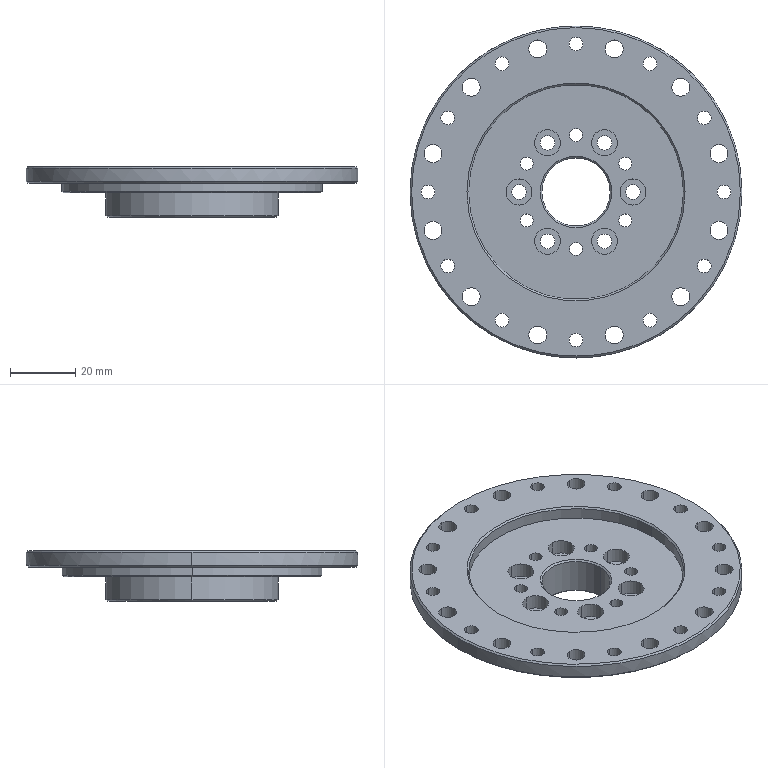NC program | NX | posted with a generic post | part box 102 x 102 x 15.5 mm
Whole program, first 1471 of 1643 lines:
N10 G17 G21 G94 G90
(FLOOR_WALL_COPY , TOOL : D80)
N12 T19 M6
N14 G54
N16 G17 G0 G90 X-84.262 Y55.699 S6500 M3
N18 G43 Z30. H19
N20 Z3.
N22 G94 G1 Z0. F1500.
N24 X-78.199
N26 X78.203
N28 G2 X89.259 Y35.357 R95.973
N30 X89.433 Y34.914 R95.942
N32 X94.701 Y15.851 R95.326
N34 G1 X-94.691
N36 G3 X-95.022 Y13.714 R94.858
N38 X-95.92 Y4.092 R95.982
N40 X-95.99 Y1.889 R94.629
N42 G1 Y-1.902
N44 G3 X-95.896 Y-4.628 R94.629
N46 X-92.96 Y-23.997 R95.982
N48 G1 X92.973
N50 X98.128
N52 Z3.
N54 G0 Z30.
N56 M5
(ADAPTIVE_MILLING , TOOL : D10)
N58 T15 M6
N60 G54
N62 G17 G0 G90 X-67.76 Y0.059 S9500 M3
N64 G43 Z30. H15
N66 Z-12.5
N68 G94 G1 Z-15.5 F1000.
N70 X-65.308 Y-1.34 F3000.
N72 G3 X-61.038 Y0.059 R3.035
N74 X-60.26 Y3.192 R10.742
N76 G2 X-58.272 Y14.714 R96.806
N78 X55.794 Y22.284 R60.088
N80 X58.924 Y11.642 R86.808
N82 X-21.027 Y-56.295 R60.049
N84 X-60.002 Y-2.912 R59.983
N86 X-59.421 Y3.257 R54.222
N88 X-56.513 Y17.745 R79.336
N90 X54.587 Y22.926 R59.214
N92 X58.538 Y8.9 R69.26
N94 X-59.012 Y-4.793 R-59.209
N96 X-58.536 Y3.583 R50.601
N98 X-54.133 Y21.8 R69.323
N100 X53.512 Y23.227 R58.336
N102 X58.008 Y6.271 R63.189
N104 X6.297 Y-58.02 R58.341
N106 X-58.005 Y-6.205 R58.341
N108 X-57.547 Y4.664 R51.864
N110 X-50.605 Y27.282 R63.438
N112 X52.533 Y23.282 R57.458
N114 X57.485 Y-0.531 R59.067
N116 X-56.992 Y-7.349 R57.474
N118 X-56.706 Y4.521 R51.402
N120 X-49.511 Y27.467 R62.441
N122 X51.543 Y23.365 R56.585
N124 X56.377 Y-5.211 R57.429
N126 X-55.921 Y-8.712 R56.604
N128 X-56.034 Y2.76 R47.908
N130 G1 X-55.954 Y4.661
N132 X-55.943 Y4.788
N134 X-55.368 Y9.322
N136 X-55.347 Y9.448
N138 X-54.395 Y13.918
N140 X-54.363 Y14.042
N142 X-53.041 Y18.417
N144 X-52.999 Y18.537
N146 X-51.316 Y22.786
N148 X-51.264 Y22.903
N150 X-49.231 Y26.996
N152 X-49.17 Y27.108
N154 X-46.802 Y31.017
N156 X-46.732 Y31.124
N158 X-44.045 Y34.821
N160 X-43.966 Y34.921
N162 X-40.98 Y38.381
N164 X-40.893 Y38.474
N166 X-37.628 Y41.673
N168 X-37.534 Y41.758
N170 X-34.013 Y44.673
N172 X-33.911 Y44.75
N174 X-30.159 Y47.36
N176 X-30.052 Y47.428
N178 X-26.095 Y49.715
N180 X-25.982 Y49.774
N182 X-21.847 Y51.722
N184 X-21.73 Y51.772
N186 X-17.447 Y53.368
N188 X-17.326 Y53.407
N190 X-12.925 Y54.64
N192 X-12.801 Y54.669
N194 X-8.312 Y55.529
N196 X-8.186 Y55.547
N198 X-3.641 Y56.029
N200 X-3.513 Y56.037
N202 X1.092 Y56.138
N204 X1.167 Y56.136
N206 X5.745 Y55.853
N208 X5.872 Y55.839
N210 X10.395 Y55.177
N212 X10.518 Y55.153
N214 X14.845 Y54.15
N216 X14.964 Y54.117
N218 X19.196 Y52.764
N220 X19.312 Y52.722
N222 X23.42 Y51.03
N224 X23.533 Y50.978
N226 X27.489 Y48.958
N228 X27.597 Y48.897
N230 X31.376 Y46.562
N232 X31.479 Y46.493
N234 X35.056 Y43.859
N236 X35.153 Y43.781
N238 X38.504 Y40.865
N240 X38.594 Y40.78
N242 X41.698 Y37.601
N244 X41.78 Y37.509
N246 X44.615 Y34.089
N248 X44.69 Y33.99
N250 X47.238 Y30.351
N252 X47.304 Y30.246
N254 X49.548 Y26.412
N256 X49.606 Y26.302
N258 X51.53 Y22.298
N260 X51.579 Y22.184
N262 X53.171 Y18.037
N264 X53.211 Y17.92
N266 X54.461 Y13.657
N268 X54.491 Y13.537
N270 X55.391 Y9.187
N272 X55.411 Y9.064
N274 X55.954 Y4.655
N276 X55.964 Y4.532
N278 X56.149 Y0.062
N280 Y0.03
N282 Y0.
N284 X55.968 Y-4.481
N286 X55.958 Y-4.605
N288 X55.417 Y-9.026
N290 X55.397 Y-9.149
N292 X54.498 Y-13.511
N294 X54.468 Y-13.632
N296 X53.216 Y-17.906
N298 X53.176 Y-18.024
N300 X51.58 Y-22.182
N302 X51.531 Y-22.296
N304 X49.602 Y-26.31
N306 X49.543 Y-26.42
N308 X47.294 Y-30.263
N310 X47.225 Y-30.369
N312 X44.58 Y-34.134
N314 X44.502 Y-34.236
N316 X41.55 Y-37.764
N318 X41.464 Y-37.859
N320 X38.225 Y-41.126
N322 X38.131 Y-41.213
N324 X34.629 Y-44.196
N326 X34.528 Y-44.276
N328 X30.788 Y-46.954
N330 X30.68 Y-47.024
N332 X26.728 Y-49.378
N334 X26.615 Y-49.438
N336 X22.479 Y-51.451
N338 X22.361 Y-51.503
N340 X18.07 Y-53.16
N342 X17.948 Y-53.201
N344 X13.533 Y-54.492
N346 X13.408 Y-54.523
N348 X8.9 Y-55.438
N350 X8.773 Y-55.458
N352 X4.204 Y-55.99
N354 X4.076 Y-55.999
N356 X-0.571 Y-56.146
N358 X-0.627 Y-56.145
N360 X-5.245 Y-55.902
N362 X-5.372 Y-55.89
N364 X-9.93 Y-55.262
N366 X-10.056 Y-55.239
N368 X-14.544 Y-54.231
N370 X-14.668 Y-54.197
N372 X-19.056 Y-52.815
N374 X-19.176 Y-52.771
N376 X-23.432 Y-51.024
N378 X-23.549 Y-50.97
N380 X-27.642 Y-48.872
N382 X-27.754 Y-48.808
N384 X-31.656 Y-46.373
N386 X-31.762 Y-46.3
N388 X-35.446 Y-43.545
N390 X-35.545 Y-43.463
N392 X-38.984 Y-40.408
N394 X-39.076 Y-40.318
N396 X-42.246 Y-36.984
N398 X-42.33 Y-36.888
N400 X-45.208 Y-33.299
N402 X-45.284 Y-33.195
N404 X-47.85 Y-29.375
N406 X-47.915 Y-29.269
N408 G2 X-51.905 Y-21.412 R65.133
N410 X-54.616 Y-13.025 R65.155
N412 X-55.982 Y-4.317 R65.155
N414 G1 X-56.149 Y0.002
N416 Y0.028
N418 Y0.063
N420 X-56.034 Y2.761
N422 G3 X-58.817 Y5.91 R3.036
N424 G1 X-62.113 Y6.176
N426 Z-12.5
N428 G0 Z30.
N430 X-4.479 Y-0.427
N432 Z3.
N434 G3 X-4.479 Y-0.427 Z2.506 I4.48 J0.423 F1000.
N436 X-4.479 Y-0.427 Z2.013 I4.48 J0.423
N438 X-4.479 Y-0.427 Z1.519 I4.48 J0.423
N440 X-4.479 Y-0.427 Z1.026 I4.48 J0.423
N442 X-4.479 Y-0.427 Z0.532 I4.48 J0.423
N444 X-4.479 Y-0.427 Z0.039 I4.48 J0.423
N446 X-4.479 Y-0.427 Z-0.455 I4.48 J0.423
N448 X-4.479 Y-0.427 Z-0.948 I4.48 J0.423
N450 X-4.479 Y-0.427 Z-1.442 I4.48 J0.423
N452 X-4.479 Y-0.427 Z-1.935 I4.48 J0.423
N454 X-4.479 Y-0.427 Z-2.429 I4.48 J0.423
N456 X-4.479 Y-0.427 Z-2.922 I4.48 J0.423
N458 X-4.479 Y-0.427 Z-3.416 I4.48 J0.423
N460 X-4.479 Y-0.427 Z-3.909 I4.48 J0.423
N462 X-4.479 Y-0.427 Z-4.403 I4.48 J0.423
N464 X-4.479 Y-0.427 Z-4.896 I4.48 J0.423
N466 X-4.479 Y-0.427 Z-5.39 I4.48 J0.423
N468 X-4.479 Y-0.427 Z-5.884 I4.48 J0.423
N470 X-4.479 Y-0.427 Z-6.377 I4.48 J0.423
N472 X-4.479 Y-0.427 Z-6.871 I4.48 J0.423
N474 X-4.479 Y-0.427 Z-7.364 I4.48 J0.423
N476 X-4.479 Y-0.427 Z-7.858 I4.48 J0.423
N478 X-4.479 Y-0.427 Z-8.351 I4.48 J0.423
N480 X-4.479 Y-0.427 Z-8.845 I4.48 J0.423
N482 X-4.479 Y-0.427 Z-9.338 I4.48 J0.423
N484 X-4.479 Y-0.427 Z-9.832 I4.48 J0.423
N486 X-4.479 Y-0.427 Z-10.325 I4.48 J0.423
N488 X-4.479 Y-0.427 Z-10.819 I4.48 J0.423
N490 X-4.479 Y-0.427 Z-11.312 I4.48 J0.423
N492 X-4.479 Y-0.427 Z-11.806 I4.48 J0.423
N494 X-4.479 Y-0.427 Z-12.299 I4.48 J0.423
N496 X-4.479 Y-0.427 Z-12.793 I4.48 J0.423
N498 X-4.479 Y-0.427 Z-13.287 I4.48 J0.423
N500 X-4.479 Y-0.427 Z-13.78 I4.48 J0.423
N502 X-4.479 Y-0.427 Z-14.274 I4.48 J0.423
N504 X-4.479 Y-0.427 Z-14.767 I4.48 J0.423
N506 X-4.479 Y-0.427 Z-15.261 I4.48 J0.423
N508 X4.501 Y-0.004 Z-15.5 R4.5
N510 X3.843 Y-2.357 R-4.5 F3000.
N512 X-1.656 Y4.571 R4.635
N514 X4.089 Y-2.695 R-4.873
N516 X-2.389 Y4.669 R5.042
N518 X4.374 Y-2.973 R-5.26
N520 G1 X4.556 Y-2.703
N522 X4.718 Y-2.42
N524 G3 X-4.21 Y-3.248 R-5.316
N526 X4.922 Y-2.007 R5.315
N528 X-0.274 Y0.993 R3.963
N530 G1 Z-12.5
N532 G0 Z30.
N534 X0.719 Y-0.017
N536 Z-0.875
N538 G1 Z-3.875 F1000.
N540 G3 X-5.281 Y-0.017 R3.28 F3000.
N542 X-5.118 Y-2.574 R3.113
N544 X5.78 Y-0.494 R5.749
N546 X-5.688 Y1.209 R5.809
N548 X-4.956 Y-3.185 R5.321
N550 X-5.873 Y0.342 R-5.885
N552 X0.127 Y0.342 R3.418
N554 G1 Z-0.875
N556 G0 Z30.
N558 X0.15 Y-0.027
N560 Z-0.849
N562 G1 Z-3.849 F1000.
N564 G3 X-5.85 Y-0.027 R3.363 F3000.
N566 X-5.793 Y-2.499 R3.12
N568 X5.487 Y-3.281 R6.314
N570 X-6.268 Y1.312 R-6.397
N572 X-1.962 Y-6.557 R6.251
N574 X-6.491 Y2.262 R-6.855
N576 X0.081 Y-7.325 R6.917
N578 X-6.628 Y3.189 R-7.338
N580 X1.216 Y-7.724 R7.476
N582 X-6.863 Y3.817 R-7.831
N584 X1.93 Y-8.097 R8.006
N586 X-7.106 Y4.408 R-8.338
N588 X2.645 Y-8.436 R8.538
N590 X-7.38 Y4.946 R-8.857
N592 X3.196 Y-8.805 R9.073
N594 X-7.529 Y5.647 R-9.384
N596 X3.994 Y-9.065 R9.62
N598 X-7.75 Y6.24 R-9.924
N600 X4.333 Y-9.513 R10.169
N602 X-7.885 Y6.931 R-10.472
N604 X4.805 Y-9.906 R10.728
N606 X-8.091 Y7.536 R-11.03
N608 X4.998 Y-10.44 R11.293
N610 X-8.266 Y8.171 R-11.595
N612 X5.584 Y-10.788 R11.867
N614 X-8.66 Y8.591 R-12.17
N616 X5.98 Y-11.236 R12.446
N618 X-8.741 Y9.323 R-12.751
N620 X6.32 Y-11.72 R13.033
N622 X-9.193 Y9.708 R-13.34
N624 X6.3 Y-12.403 R13.626
N626 X-9.479 Y10.257 R-13.937
N628 X6.943 Y-12.743 R14.227
N630 X-9.712 Y10.861 R-14.539
N632 X7.242 Y-13.274 R14.834
N634 X-9.934 Y11.477 R-15.148
N636 X7.687 Y-13.728 R15.446
N638 X-10.27 Y12.001 R-15.763
N640 X8.074 Y-14.221 R16.064
N642 X-10.464 Y12.649 R-16.383
N644 X8.544 Y-14.67 R16.689
N646 X-10.639 Y13.313 R-17.008
N648 X8.981 Y-15.143 R17.318
N650 X-10.929 Y13.89 R-17.639
N652 X8.929 Y-15.907 R17.951
N654 X-10.992 Y14.641 R-18.274
N656 X9.137 Y-16.523 R18.589
N658 X-11.366 Y15.164 R-18.915
N660 X9.411 Y-17.107 R19.231
N662 X-11.466 Y15.89 R-19.559
N664 X9.463 Y-17.814 R19.878
N666 X-11.755 Y16.481 R-20.207
N668 X10.237 Y-18.133 R20.529
N670 X-12.133 Y17.014 R-20.859
N672 X10.129 Y-18.937 R21.181
N674 X-12.169 Y17.788 R-21.513
N676 X10.791 Y-19.329 R21.841
N678 X-12.753 Y18.188 R-22.174
N680 X11.145 Y-19.888 R22.502
N682 X-13.04 Y18.796 R-22.836
N684 X11.527 Y-20.437 R23.166
N686 X-13.178 Y19.509 R-23.503
N688 X12.09 Y-20.884 R23.834
N690 X-13.23 Y20.278 R-24.172
N692 X12.035 Y-21.69 R24.506
N694 X-13.26 Y21.056 R-24.844
N696 X12.301 Y-22.313 R25.179
N698 X-13.426 Y21.749 R-25.519
N700 X12.264 Y-23.105 R25.856
N702 X-13.886 Y22.263 R-26.198
N704 X12.697 Y-23.644 R26.535
N706 X-13.684 Y23.179 R-26.877
N708 X12.883 Y-24.319 R27.217
N710 X-13.746 Y23.935 R-27.56
N712 X-27.153 Y-6.154 R27.676
N714 X-23.732 Y-14.556 R29.482
N716 X-19.628 Y-19.743 R31.594
N718 X-14.423 Y-23.812 R31.545
N720 X-8.406 Y-26.54 R31.545
N722 X-1.916 Y-27.774 R31.545
N724 X4.682 Y-27.443 R31.384
N726 X11.017 Y-25.567 R31.545
N728 X16.731 Y-22.252 R31.545
N730 X21.503 Y-17.683 R31.545
N732 X25.019 Y-12.212 R31.66
N734 X27.678 Y-3. R29.654
N736 X27.633 Y3.393 R31.06
N738 X24.866 Y12.52 R29.643
N740 X19.181 Y20.178 R29.643
N742 X11.245 Y25.468 R29.643
N744 X1.909 Y27.774 R29.599
N746 X-4.609 Y27.456 R31.347
N748 X-13.491 Y24.353 R29.846
N750 X-21.301 Y17.926 R29.418
N752 X-26.055 Y9.807 R29.846
N754 X-27.665 Y3.116 R30.899
N756 G1 X-27.84 Y0.204
N758 X-27.845 Y0.021
N760 X-27.841 Y-0.142
N762 X-27.697 Y-2.833
N764 X-27.686 Y-2.932
N766 G3 X-23.713 Y-5.48 R3.034
N768 G1 X-21.034 Y-4.584
N770 Z-0.849
N772 G0 Z30.
N774 M5
(ZLEVEL_PROFILE_COPY_1_COPY_COPY_1 , TOOL : D10JING)
N776 T14 M6
N778 G54
N780 G17 G0 G90 X-57.975 Y-1.717 S9500 M3
N782 G43 Z30. H14
N784 Z-14.5
N786 G94 G1 Z-15.5 F1000.
N788 X-56.5 Y-0.866
N790 G3 X-56. Y0. R1.
N792 G1 Y0.024 F1200.
N794 G2 X0.024 Y56. R56.
N796 X-56. Y0. R-56.
N798 G3 X-56.5 Y0.866 R1.
N800 G1 X-57.975 Y1.717
N802 Z-14.5
N804 G0 Z30.
(ZLEVEL_PROFILE_COPY_1_COPY_COPY_1_COPY , TOOL : D10JING)
N806 X-2.75 Y2.165
N808 Z-14.5
N810 G1 Z-15.5 F1000.
N812 X-5. Y0.866
N814 G3 X-5.5 Y0. R1.
N816 X0. Y-5.5 R5.5 F1200.
N818 X-5.5 Y0. R-5.5
N820 X-5. Y-0.866 R1.
N822 G1 X-2.75 Y-2.165
N824 Z-14.5
N826 G0 Z30.
(FLOOR_WALL_COPY_1_COPY , TOOL : D10JING)
N828 X0.6 Y0.
N830 Z-1.
N832 G1 Z-4. F1000.
N834 X-2.4
N836 G3 X-0.277 Y2.384 R-2.4 F1200.
N838 X-1.405 Y1.92 R2.25
N840 G1 X-5.519 Y-1.306
N842 G3 X-5.935 Y-4.42 R2.25
N844 X-6.809 Y2.898 R-7.4
N846 G2 X-7.382 Y2.071 R2.5
N848 G1 X-11.074 Y-1.456
N850 G3 X-11.707 Y-4.087 R2.5
N852 X-11.999 Y3.128 R-12.4
N854 G2 X-12.667 Y1.975 R2.5
N856 G1 X-16.271 Y-1.56
N858 G3 X-16.956 Y-3.905 R2.5
N860 X-17.097 Y3.235 R-17.4
N862 G2 X-17.794 Y1.924 R2.5
N864 G1 X-21.368 Y-1.612
N866 G3 X-22.073 Y-3.814 R2.5
N868 X-22.156 Y3.298 R-22.4
N870 G2 X-22.866 Y1.893 R2.5
N872 G1 X-26.427 Y-1.643
N874 G3 X-27.141 Y-3.759 R2.5
N876 X-27.141 Y-3.759 R-27.4
N878 X-26.945 Y-4.972 R27.4
N880 G1 X-23.995 Y-4.428
N882 X-27.437 Y-5.063 F1000.
N884 G3 X5.063 Y-27.437 R27.9 F1200.
N886 X-27.437 Y-5.063 R-27.9
N888 G1 X-24.487 Y-4.519
N890 Z-1.
N892 G0 Z30.
N894 M5
(DRILLING_COPY_1 , TOOL : D6A45)
N896 T01 M6
N898 G54
N900 G17 G0 G90 X0. Y0. S5000 M3
N902 G43 Z30. H1
N904 G94 G81 G98 Z-1. F350. R3.
N906 Y-17.5 Z-5. R-1.
N908 X8.75 Y-15.155
N910 X15.155 Y-8.75
N912 X17.5 Y0.
N914 X15.155 Y8.75
N916 X8.75 Y15.155
N918 X0. Y17.5
N920 X-8.75 Y15.155
N922 X-15.155 Y8.75
N924 X-17.5 Y0.
N926 X-15.155 Y-8.75
N928 X-8.75 Y-15.155
N930 X-22.75 Y-39.404 Z-1. R3.
N932 X-11.776 Y-43.95
N934 X0. Y-45.5
N936 X11.776 Y-43.95
N938 X22.75 Y-39.404
N940 X32.173 Y-32.173
N942 X39.404 Y-22.75
N944 X43.95 Y-11.776
N946 X45.5 Y0.
N948 X43.95 Y11.776
N950 X39.404 Y22.75
N952 X32.173 Y32.173
N954 X22.75 Y39.404
N956 X11.776 Y43.95
N958 X0. Y45.5
N960 X-11.776 Y43.95
N962 X-22.75 Y39.404
N964 X-32.173 Y32.173
N966 X-39.404 Y22.75
N968 X-43.95 Y11.776
N970 X-45.5 Y0.
N972 X-43.95 Y-11.776
N974 X-39.404 Y-22.75
N976 X-32.173 Y-32.173
N978 G80
N980 G0 X-32.173 Y-32.173 Z30.
N982 M5
(DRILLING_COPY_COPY_COPY_2_COPY , TOOL : 4.2ZT)
N984 T04 M6
N986 G54
N988 G17 G0 G90 X-22.75 Y-39.404 S2000 M3
N990 G43 Z30. H4
N992 G94 G83 G98 Z-7.762 F180. Q2. R3.
N994 X-39.404 Y-22.75
N996 X-45.5 Y0.
N998 X-39.404 Y22.75
N1000 X-22.75 Y39.404
N1002 X0. Y45.5
N1004 X22.75 Y39.404
N1006 X39.404 Y22.75
N1008 X45.5 Y0.
N1010 X39.404 Y-22.75
N1012 X22.75 Y-39.404
N1014 X0. Y-45.5
N1016 G80
N1018 G0 X0. Y-45.5 Z30.
N1020 M5
(DRILLING_COPY_COPY_COPY_2_COPY_COPY , TOOL : 5.5ZT)
N1022 T09 M6
N1024 G54
N1026 G17 G0 G90 X32.173 Y32.173 S2000 M3
N1028 G43 Z30. H9
N1030 G94 G83 G98 Z-8.152 F180. Q2. R3.
N1032 X11.776 Y43.95
N1034 X-11.776
N1036 X-32.173 Y32.173
N1038 X-43.95 Y11.776
N1040 Y-11.776
N1042 X-32.173 Y-32.173
N1044 X-11.776 Y-43.95
N1046 X11.776
N1048 X32.173 Y-32.173
N1050 X43.95 Y-11.776
N1052 Y11.776
N1054 G80
N1056 G0 X43.95 Y11.776 Z30.
N1058 M5
(DRILLING_COPY_COPY_COPY_2 , TOOL : 4.5ZT)
N1060 T08 M6
N1062 G54
N1064 G17 G0 G90 X-8.75 Y15.155 S2000 M3
N1066 G43 Z30. H8
N1068 G94 G83 G98 Z-18.352 F180. Q2. R-1.
N1070 X8.75
N1072 X17.5 Y0.
N1074 X8.75 Y-15.155
N1076 X-8.75
N1078 X-17.5 Y0.
N1080 G80
N1082 G0 X-17.5 Y0. Z30.
N1084 M5
(DRILLING_COPY_COPY_COPY_2_COPY_1 , TOOL : 3.5ZT)
N1086 T07 M6
N1088 G54
N1090 G17 G0 G90 X0. Y17.5 S2000 M3
N1092 G43 Z30. H7
N1094 G94 G83 G98 Z-18.052 F180. Q2. R-1.
N1096 X15.155 Y8.75
N1098 Y-8.75
N1100 X0. Y-17.5
N1102 X-15.155 Y-8.75
N1104 Y8.75
N1106 G80
N1108 G0 X-15.155 Y8.75 Z30.
N1110 M5
(HOLE_MILLING , TOOL : D6)
N1112 T12 M6
N1114 G54
N1116 G17 G0 G90 X8.75 Y15.155 S9500 M3
N1118 G43 Z30. H12
N1120 Z-3.5
N1122 G94 G3 X9.25 Y14.655 R0.5 F1400.
N1124 X9.75 Y15.155 R0.5
N1126 X9.75 Y15.155 Z-3.9 I-1. J0.
N1128 X9.75 Y15.155 Z-4.3 I-1. J0.
N1130 X9.75 Y15.155 Z-4.7 I-1. J0.
N1132 X9.75 Y15.155 Z-5.1 I-1. J0.
N1134 X9.75 Y15.155 Z-5.5 I-1. J0.
N1136 X9.75 Y15.155 Z-5.9 I-1. J0.
N1138 X9.75 Y15.155 Z-6.3 I-1. J0.
N1140 X9.75 Y15.155 Z-6.7 I-1. J0.
N1142 X9.75 Y15.155 Z-7.1 I-1. J0.
N1144 X9.75 Y15.155 Z-7.5 I-1. J0.
N1146 X9.75 Y15.155 Z-7.9 I-1. J0.
N1148 X9.75 Y15.155 Z-8.3 I-1. J0.
N1150 X8.75 Y14.155 Z-8.6 R-1.
N1152 X9.75 Y15.155 R1.
N1154 X8.75 Y14.155 R-1.
N1156 X9.25 Y14.655 R0.5
N1158 X8.75 Y15.155 R0.5
N1160 G0 Z30.
N1162 X17.5 Y0.
N1164 Z-3.5
N1166 G3 X18. Y-0.5 R0.5
N1168 X18.5 Y0. R0.5
N1170 X18.5 Y0. Z-3.9 I-1. J0.
N1172 X18.5 Y0. Z-4.3 I-1. J0.
N1174 X18.5 Y0. Z-4.7 I-1. J0.
N1176 X18.5 Y0. Z-5.1 I-1. J0.
N1178 X18.5 Y0. Z-5.5 I-1. J0.
N1180 X18.5 Y0. Z-5.9 I-1. J0.
N1182 X18.5 Y0. Z-6.3 I-1. J0.
N1184 X18.5 Y0. Z-6.7 I-1. J0.
N1186 X18.5 Y0. Z-7.1 I-1. J0.
N1188 X18.5 Y0. Z-7.5 I-1. J0.
N1190 X18.5 Y0. Z-7.9 I-1. J0.
N1192 X18.5 Y0. Z-8.3 I-1. J0.
N1194 X17.5 Y-1. Z-8.6 R-1.
N1196 X18.5 Y0. R1.
N1198 X17.5 Y-1. R-1.
N1200 X18. Y-0.5 R0.5
N1202 X17.5 Y0. R0.5
N1204 G0 Z30.
N1206 X8.75 Y-15.155
N1208 Z-3.5
N1210 G3 X9.25 Y-15.655 R0.5
N1212 X9.75 Y-15.155 R0.5
N1214 X9.75 Y-15.155 Z-3.9 I-1. J0.
N1216 X9.75 Y-15.155 Z-4.3 I-1. J0.
N1218 X9.75 Y-15.155 Z-4.7 I-1. J0.
N1220 X9.75 Y-15.155 Z-5.1 I-1. J0.
N1222 X9.75 Y-15.155 Z-5.5 I-1. J0.
N1224 X9.75 Y-15.155 Z-5.9 I-1. J0.
N1226 X9.75 Y-15.155 Z-6.3 I-1. J0.
N1228 X9.75 Y-15.155 Z-6.7 I-1. J0.
N1230 X9.75 Y-15.155 Z-7.1 I-1. J0.
N1232 X9.75 Y-15.155 Z-7.5 I-1. J0.
N1234 X9.75 Y-15.155 Z-7.9 I-1. J0.
N1236 X9.75 Y-15.155 Z-8.3 I-1. J0.
N1238 X8.75 Y-16.155 Z-8.6 R-1.
N1240 X9.75 Y-15.155 R1.
N1242 X8.75 Y-16.155 R-1.
N1244 X9.25 Y-15.655 R0.5
N1246 X8.75 Y-15.155 R0.5
N1248 G0 Z30.
N1250 X-8.75
N1252 Z-3.5
N1254 G3 X-8.25 Y-15.655 R0.5
N1256 X-7.75 Y-15.155 R0.5
N1258 X-7.75 Y-15.155 Z-3.9 I-1. J0.
N1260 X-7.75 Y-15.155 Z-4.3 I-1. J0.
N1262 X-7.75 Y-15.155 Z-4.7 I-1. J0.
N1264 X-7.75 Y-15.155 Z-5.1 I-1. J0.
N1266 X-7.75 Y-15.155 Z-5.5 I-1. J0.
N1268 X-7.75 Y-15.155 Z-5.9 I-1. J0.
N1270 X-7.75 Y-15.155 Z-6.3 I-1. J0.
N1272 X-7.75 Y-15.155 Z-6.7 I-1. J0.
N1274 X-7.75 Y-15.155 Z-7.1 I-1. J0.
N1276 X-7.75 Y-15.155 Z-7.5 I-1. J0.
N1278 X-7.75 Y-15.155 Z-7.9 I-1. J0.
N1280 X-7.75 Y-15.155 Z-8.3 I-1. J0.
N1282 X-8.75 Y-16.155 Z-8.6 R-1.
N1284 X-7.75 Y-15.155 R1.
N1286 X-8.75 Y-16.155 R-1.
N1288 X-8.25 Y-15.655 R0.5
N1290 X-8.75 Y-15.155 R0.5
N1292 G0 Z30.
N1294 X-17.5 Y0.
N1296 Z-3.5
N1298 G3 X-17. Y-0.5 R0.5
N1300 X-16.5 Y0. R0.5
N1302 X-16.5 Y0. Z-3.9 I-1. J0.
N1304 X-16.5 Y0. Z-4.3 I-1. J0.
N1306 X-16.5 Y0. Z-4.7 I-1. J0.
N1308 X-16.5 Y0. Z-5.1 I-1. J0.
N1310 X-16.5 Y0. Z-5.5 I-1. J0.
N1312 X-16.5 Y0. Z-5.9 I-1. J0.
N1314 X-16.5 Y0. Z-6.3 I-1. J0.
N1316 X-16.5 Y0. Z-6.7 I-1. J0.
N1318 X-16.5 Y0. Z-7.1 I-1. J0.
N1320 X-16.5 Y0. Z-7.5 I-1. J0.
N1322 X-16.5 Y0. Z-7.9 I-1. J0.
N1324 X-16.5 Y0. Z-8.3 I-1. J0.
N1326 X-17.5 Y-1. Z-8.6 R-1.
N1328 X-16.5 Y0. R1.
N1330 X-17.5 Y-1. R-1.
N1332 X-17. Y-0.5 R0.5
N1334 X-17.5 Y0. R0.5
N1336 G0 Z30.
N1338 X-8.75 Y15.155
N1340 Z-3.5
N1342 G3 X-8.25 Y14.655 R0.5
N1344 X-7.75 Y15.155 R0.5
N1346 X-7.75 Y15.155 Z-3.9 I-1. J0.
N1348 X-7.75 Y15.155 Z-4.3 I-1. J0.
N1350 X-7.75 Y15.155 Z-4.7 I-1. J0.
N1352 X-7.75 Y15.155 Z-5.1 I-1. J0.
N1354 X-7.75 Y15.155 Z-5.5 I-1. J0.
N1356 X-7.75 Y15.155 Z-5.9 I-1. J0.
N1358 X-7.75 Y15.155 Z-6.3 I-1. J0.
N1360 X-7.75 Y15.155 Z-6.7 I-1. J0.
N1362 X-7.75 Y15.155 Z-7.1 I-1. J0.
N1364 X-7.75 Y15.155 Z-7.5 I-1. J0.
N1366 X-7.75 Y15.155 Z-7.9 I-1. J0.
N1368 X-7.75 Y15.155 Z-8.3 I-1. J0.
N1370 X-8.75 Y14.155 Z-8.6 R-1.
N1372 X-7.75 Y15.155 R1.
N1374 X-8.75 Y14.155 R-1.
N1376 X-8.25 Y14.655 R0.5
N1378 X-8.75 Y15.155 R0.5
N1380 G0 Z30.
N1382 M5
(HOLE_MILLING_COPY , TOOL : D3)
N1384 T16 M6
N1386 G54
N1388 G17 G0 G90 X0. Y17.5 S9500 M3
N1390 G43 Z30. H16
N1392 Z-3.5
N1394 G94 G3 X0.22 Y17.28 R0.22 F1200.
N1396 X0.44 Y17.5 R0.22
N1398 X0.44 Y17.5 Z-3.8 I-0.44 J0.
N1400 X0.44 Y17.5 Z-4.1 I-0.44 J0.
N1402 X0.44 Y17.5 Z-4.4 I-0.44 J0.
N1404 X0.44 Y17.5 Z-4.7 I-0.44 J0.
N1406 X0.44 Y17.5 Z-5. I-0.44 J0.
N1408 X0.44 Y17.5 Z-5.3 I-0.44 J0.
N1410 X0.44 Y17.5 Z-5.6 I-0.44 J0.
N1412 X0.44 Y17.5 Z-5.9 I-0.44 J0.
N1414 X0.44 Y17.5 Z-6.2 I-0.44 J0.
N1416 X0.44 Y17.5 Z-6.5 I-0.44 J0.
N1418 X0.44 Y17.5 Z-6.8 I-0.44 J0.
N1420 X0.44 Y17.5 Z-7.1 I-0.44 J0.
N1422 X0.44 Y17.5 Z-7.4 I-0.44 J0.
N1424 X0.44 Y17.5 Z-7.7 I-0.44 J0.
N1426 X0.44 Y17.5 Z-8. I-0.44 J0.
N1428 X0.44 Y17.5 Z-8.3 I-0.44 J0.
N1430 X0.44 Y17.5 Z-8.6 I-0.44 J0.
N1432 X0.44 Y17.5 Z-8.9 I-0.44 J0.
N1434 X0.44 Y17.5 Z-9.2 I-0.44 J0.
N1436 X0.44 Y17.5 Z-9.5 I-0.44 J0.
N1438 X0.44 Y17.5 Z-9.8 I-0.44 J0.
N1440 X0.44 Y17.5 Z-10.1 I-0.44 J0.
N1442 X0.44 Y17.5 Z-10.4 I-0.44 J0.
N1444 X0.44 Y17.5 Z-10.7 I-0.44 J0.
N1446 X0.44 Y17.5 Z-11. I-0.44 J0.
N1448 X0.44 Y17.5 Z-11.3 I-0.44 J0.
N1450 X0.44 Y17.5 Z-11.6 I-0.44 J0.
N1452 X0.44 Y17.5 Z-11.9 I-0.44 J0.
N1454 X0.44 Y17.5 Z-12.2 I-0.44 J0.
N1456 X0.44 Y17.5 Z-12.5 I-0.44 J0.
N1458 X0.44 Y17.5 Z-12.8 I-0.44 J0.
N1460 X0.44 Y17.5 Z-13.1 I-0.44 J0.
N1462 X0.44 Y17.5 Z-13.4 I-0.44 J0.
N1464 X0.44 Y17.5 Z-13.7 I-0.44 J0.
N1466 X0.44 Y17.5 Z-14. I-0.44 J0.
N1468 X0.44 Y17.5 Z-14.3 I-0.44 J0.
N1470 X0.44 Y17.5 Z-14.6 I-0.44 J0.
N1472 X0.44 Y17.5 Z-14.9 I-0.44 J0.
N1474 X0.44 Y17.5 Z-15.2 I-0.44 J0.
N1476 X0.44 Y17.5 Z-15.5 I-0.44 J0.
N1478 X0. Y17.94 R0.44
N1480 X0.44 Y17.5 R-0.44
N1482 X0.22 Y17.72 R0.22
N1484 X0. Y17.5 R0.22
N1486 G0 Z30.
N1488 X15.155 Y8.75
N1490 Z-3.5
N1492 G3 X15.375 Y8.53 R0.22
N1494 X15.595 Y8.75 R0.22
N1496 X15.595 Y8.75 Z-3.8 I-0.44 J0.
N1498 X15.595 Y8.75 Z-4.1 I-0.44 J0.
N1500 X15.595 Y8.75 Z-4.4 I-0.44 J0.
N1502 X15.595 Y8.75 Z-4.7 I-0.44 J0.
N1504 X15.595 Y8.75 Z-5. I-0.44 J0.
N1506 X15.595 Y8.75 Z-5.3 I-0.44 J0.
N1508 X15.595 Y8.75 Z-5.6 I-0.44 J0.
N1510 X15.595 Y8.75 Z-5.9 I-0.44 J0.
N1512 X15.595 Y8.75 Z-6.2 I-0.44 J0.
N1514 X15.595 Y8.75 Z-6.5 I-0.44 J0.
N1516 X15.595 Y8.75 Z-6.8 I-0.44 J0.
N1518 X15.595 Y8.75 Z-7.1 I-0.44 J0.
N1520 X15.595 Y8.75 Z-7.4 I-0.44 J0.
N1522 X15.595 Y8.75 Z-7.7 I-0.44 J0.
N1524 X15.595 Y8.75 Z-8. I-0.44 J0.
N1526 X15.595 Y8.75 Z-8.3 I-0.44 J0.
N1528 X15.595 Y8.75 Z-8.6 I-0.44 J0.
N1530 X15.595 Y8.75 Z-8.9 I-0.44 J0.
N1532 X15.595 Y8.75 Z-9.2 I-0.44 J0.
N1534 X15.595 Y8.75 Z-9.5 I-0.44 J0.
N1536 X15.595 Y8.75 Z-9.8 I-0.44 J0.
N1538 X15.595 Y8.75 Z-10.1 I-0.44 J0.
N1540 X15.595 Y8.75 Z-10.4 I-0.44 J0.
N1542 X15.595 Y8.75 Z-10.7 I-0.44 J0.
N1544 X15.595 Y8.75 Z-11. I-0.44 J0.
N1546 X15.595 Y8.75 Z-11.3 I-0.44 J0.
N1548 X15.595 Y8.75 Z-11.6 I-0.44 J0.
N1550 X15.595 Y8.75 Z-11.9 I-0.44 J0.
N1552 X15.595 Y8.75 Z-12.2 I-0.44 J0.
N1554 X15.595 Y8.75 Z-12.5 I-0.44 J0.
N1556 X15.595 Y8.75 Z-12.8 I-0.44 J0.
N1558 X15.595 Y8.75 Z-13.1 I-0.44 J0.
N1560 X15.595 Y8.75 Z-13.4 I-0.44 J0.
N1562 X15.595 Y8.75 Z-13.7 I-0.44 J0.
N1564 X15.595 Y8.75 Z-14. I-0.44 J0.
N1566 X15.595 Y8.75 Z-14.3 I-0.44 J0.
N1568 X15.595 Y8.75 Z-14.6 I-0.44 J0.
N1570 X15.595 Y8.75 Z-14.9 I-0.44 J0.
N1572 X15.595 Y8.75 Z-15.2 I-0.44 J0.
N1574 X15.595 Y8.75 Z-15.5 I-0.44 J0.
N1576 X15.155 Y9.19 R0.44
N1578 X15.595 Y8.75 R-0.44
N1580 X15.375 Y8.97 R0.22
N1582 X15.155 Y8.75 R0.22
N1584 G0 Z30.
N1586 Y-8.75
N1588 Z-3.5
N1590 G3 X15.375 Y-8.97 R0.22
N1592 X15.595 Y-8.75 R0.22
N1594 X15.595 Y-8.75 Z-3.8 I-0.44 J0.
N1596 X15.595 Y-8.75 Z-4.1 I-0.44 J0.
N1598 X15.595 Y-8.75 Z-4.4 I-0.44 J0.
N1600 X15.595 Y-8.75 Z-4.7 I-0.44 J0.
N1602 X15.595 Y-8.75 Z-5. I-0.44 J0.
N1604 X15.595 Y-8.75 Z-5.3 I-0.44 J0.
N1606 X15.595 Y-8.75 Z-5.6 I-0.44 J0.
N1608 X15.595 Y-8.75 Z-5.9 I-0.44 J0.
N1610 X15.595 Y-8.75 Z-6.2 I-0.44 J0.
N1612 X15.595 Y-8.75 Z-6.5 I-0.44 J0.
N1614 X15.595 Y-8.75 Z-6.8 I-0.44 J0.
N1616 X15.595 Y-8.75 Z-7.1 I-0.44 J0.
N1618 X15.595 Y-8.75 Z-7.4 I-0.44 J0.
N1620 X15.595 Y-8.75 Z-7.7 I-0.44 J0.
N1622 X15.595 Y-8.75 Z-8. I-0.44 J0.
N1624 X15.595 Y-8.75 Z-8.3 I-0.44 J0.
N1626 X15.595 Y-8.75 Z-8.6 I-0.44 J0.
N1628 X15.595 Y-8.75 Z-8.9 I-0.44 J0.
N1630 X15.595 Y-8.75 Z-9.2 I-0.44 J0.
N1632 X15.595 Y-8.75 Z-9.5 I-0.44 J0.
N1634 X15.595 Y-8.75 Z-9.8 I-0.44 J0.
N1636 X15.595 Y-8.75 Z-10.1 I-0.44 J0.
N1638 X15.595 Y-8.75 Z-10.4 I-0.44 J0.
N1640 X15.595 Y-8.75 Z-10.7 I-0.44 J0.
N1642 X15.595 Y-8.75 Z-11. I-0.44 J0.
N1644 X15.595 Y-8.75 Z-11.3 I-0.44 J0.
N1646 X15.595 Y-8.75 Z-11.6 I-0.44 J0.
N1648 X15.595 Y-8.75 Z-11.9 I-0.44 J0.
N1650 X15.595 Y-8.75 Z-12.2 I-0.44 J0.
N1652 X15.595 Y-8.75 Z-12.5 I-0.44 J0.
N1654 X15.595 Y-8.75 Z-12.8 I-0.44 J0.
N1656 X15.595 Y-8.75 Z-13.1 I-0.44 J0.
N1658 X15.595 Y-8.75 Z-13.4 I-0.44 J0.
N1660 X15.595 Y-8.75 Z-13.7 I-0.44 J0.
N1662 X15.595 Y-8.75 Z-14. I-0.44 J0.
N1664 X15.595 Y-8.75 Z-14.3 I-0.44 J0.
N1666 X15.595 Y-8.75 Z-14.6 I-0.44 J0.
N1668 X15.595 Y-8.75 Z-14.9 I-0.44 J0.
N1670 X15.595 Y-8.75 Z-15.2 I-0.44 J0.
N1672 X15.595 Y-8.75 Z-15.5 I-0.44 J0.
N1674 X15.155 Y-8.31 R0.44
N1676 X15.595 Y-8.75 R-0.44
N1678 X15.375 Y-8.53 R0.22
N1680 X15.155 Y-8.75 R0.22
N1682 G0 Z30.
N1684 X0. Y-17.5
N1686 Z-3.5
N1688 G3 X0.22 Y-17.72 R0.22
N1690 X0.44 Y-17.5 R0.22
N1692 X0.44 Y-17.5 Z-3.8 I-0.44 J0.
N1694 X0.44 Y-17.5 Z-4.1 I-0.44 J0.
N1696 X0.44 Y-17.5 Z-4.4 I-0.44 J0.
N1698 X0.44 Y-17.5 Z-4.7 I-0.44 J0.
N1700 X0.44 Y-17.5 Z-5. I-0.44 J0.
N1702 X0.44 Y-17.5 Z-5.3 I-0.44 J0.
N1704 X0.44 Y-17.5 Z-5.6 I-0.44 J0.
N1706 X0.44 Y-17.5 Z-5.9 I-0.44 J0.
N1708 X0.44 Y-17.5 Z-6.2 I-0.44 J0.
N1710 X0.44 Y-17.5 Z-6.5 I-0.44 J0.
N1712 X0.44 Y-17.5 Z-6.8 I-0.44 J0.
N1714 X0.44 Y-17.5 Z-7.1 I-0.44 J0.
N1716 X0.44 Y-17.5 Z-7.4 I-0.44 J0.
N1718 X0.44 Y-17.5 Z-7.7 I-0.44 J0.
N1720 X0.44 Y-17.5 Z-8. I-0.44 J0.
N1722 X0.44 Y-17.5 Z-8.3 I-0.44 J0.
N1724 X0.44 Y-17.5 Z-8.6 I-0.44 J0.
N1726 X0.44 Y-17.5 Z-8.9 I-0.44 J0.
N1728 X0.44 Y-17.5 Z-9.2 I-0.44 J0.
N1730 X0.44 Y-17.5 Z-9.5 I-0.44 J0.
N1732 X0.44 Y-17.5 Z-9.8 I-0.44 J0.
N1734 X0.44 Y-17.5 Z-10.1 I-0.44 J0.
N1736 X0.44 Y-17.5 Z-10.4 I-0.44 J0.
N1738 X0.44 Y-17.5 Z-10.7 I-0.44 J0.
N1740 X0.44 Y-17.5 Z-11. I-0.44 J0.
N1742 X0.44 Y-17.5 Z-11.3 I-0.44 J0.
N1744 X0.44 Y-17.5 Z-11.6 I-0.44 J0.
N1746 X0.44 Y-17.5 Z-11.9 I-0.44 J0.
N1748 X0.44 Y-17.5 Z-12.2 I-0.44 J0.
N1750 X0.44 Y-17.5 Z-12.5 I-0.44 J0.
N1752 X0.44 Y-17.5 Z-12.8 I-0.44 J0.
N1754 X0.44 Y-17.5 Z-13.1 I-0.44 J0.
N1756 X0.44 Y-17.5 Z-13.4 I-0.44 J0.
N1758 X0.44 Y-17.5 Z-13.7 I-0.44 J0.
N1760 X0.44 Y-17.5 Z-14. I-0.44 J0.
N1762 X0.44 Y-17.5 Z-14.3 I-0.44 J0.
N1764 X0.44 Y-17.5 Z-14.6 I-0.44 J0.
N1766 X0.44 Y-17.5 Z-14.9 I-0.44 J0.
N1768 X0.44 Y-17.5 Z-15.2 I-0.44 J0.
N1770 X0.44 Y-17.5 Z-15.5 I-0.44 J0.
N1772 X0. Y-17.06 R0.44
N1774 X0.44 Y-17.5 R-0.44
N1776 X0.22 Y-17.28 R0.22
N1778 X0. Y-17.5 R0.22
N1780 G0 Z30.
N1782 X-15.155 Y-8.75
N1784 Z-3.5
N1786 G3 X-14.935 Y-8.97 R0.22
N1788 X-14.715 Y-8.75 R0.22
N1790 X-14.715 Y-8.75 Z-3.8 I-0.44 J0.
N1792 X-14.715 Y-8.75 Z-4.1 I-0.44 J0.
N1794 X-14.715 Y-8.75 Z-4.4 I-0.44 J0.
N1796 X-14.715 Y-8.75 Z-4.7 I-0.44 J0.
N1798 X-14.715 Y-8.75 Z-5. I-0.44 J0.
N1800 X-14.715 Y-8.75 Z-5.3 I-0.44 J0.
N1802 X-14.715 Y-8.75 Z-5.6 I-0.44 J0.
N1804 X-14.715 Y-8.75 Z-5.9 I-0.44 J0.
N1806 X-14.715 Y-8.75 Z-6.2 I-0.44 J0.
N1808 X-14.715 Y-8.75 Z-6.5 I-0.44 J0.
N1810 X-14.715 Y-8.75 Z-6.8 I-0.44 J0.
N1812 X-14.715 Y-8.75 Z-7.1 I-0.44 J0.
N1814 X-14.715 Y-8.75 Z-7.4 I-0.44 J0.
N1816 X-14.715 Y-8.75 Z-7.7 I-0.44 J0.
N1818 X-14.715 Y-8.75 Z-8. I-0.44 J0.
N1820 X-14.715 Y-8.75 Z-8.3 I-0.44 J0.
N1822 X-14.715 Y-8.75 Z-8.6 I-0.44 J0.
N1824 X-14.715 Y-8.75 Z-8.9 I-0.44 J0.
N1826 X-14.715 Y-8.75 Z-9.2 I-0.44 J0.
N1828 X-14.715 Y-8.75 Z-9.5 I-0.44 J0.
N1830 X-14.715 Y-8.75 Z-9.8 I-0.44 J0.
N1832 X-14.715 Y-8.75 Z-10.1 I-0.44 J0.
N1834 X-14.715 Y-8.75 Z-10.4 I-0.44 J0.
N1836 X-14.715 Y-8.75 Z-10.7 I-0.44 J0.
N1838 X-14.715 Y-8.75 Z-11. I-0.44 J0.
N1840 X-14.715 Y-8.75 Z-11.3 I-0.44 J0.
N1842 X-14.715 Y-8.75 Z-11.6 I-0.44 J0.
N1844 X-14.715 Y-8.75 Z-11.9 I-0.44 J0.
N1846 X-14.715 Y-8.75 Z-12.2 I-0.44 J0.
N1848 X-14.715 Y-8.75 Z-12.5 I-0.44 J0.
N1850 X-14.715 Y-8.75 Z-12.8 I-0.44 J0.
N1852 X-14.715 Y-8.75 Z-13.1 I-0.44 J0.
N1854 X-14.715 Y-8.75 Z-13.4 I-0.44 J0.
N1856 X-14.715 Y-8.75 Z-13.7 I-0.44 J0.
N1858 X-14.715 Y-8.75 Z-14. I-0.44 J0.
N1860 X-14.715 Y-8.75 Z-14.3 I-0.44 J0.
N1862 X-14.715 Y-8.75 Z-14.6 I-0.44 J0.
N1864 X-14.715 Y-8.75 Z-14.9 I-0.44 J0.
N1866 X-14.715 Y-8.75 Z-15.2 I-0.44 J0.
N1868 X-14.715 Y-8.75 Z-15.5 I-0.44 J0.
N1870 X-15.155 Y-8.31 R0.44
N1872 X-14.715 Y-8.75 R-0.44
N1874 X-14.935 Y-8.53 R0.22
N1876 X-15.155 Y-8.75 R0.22
N1878 G0 Z30.
N1880 Y8.75
N1882 Z-3.5
N1884 G3 X-14.935 Y8.53 R0.22
N1886 X-14.715 Y8.75 R0.22
N1888 X-14.715 Y8.75 Z-3.8 I-0.44 J0.
N1890 X-14.715 Y8.75 Z-4.1 I-0.44 J0.
N1892 X-14.715 Y8.75 Z-4.4 I-0.44 J0.
N1894 X-14.715 Y8.75 Z-4.7 I-0.44 J0.
N1896 X-14.715 Y8.75 Z-5. I-0.44 J0.
N1898 X-14.715 Y8.75 Z-5.3 I-0.44 J0.
N1900 X-14.715 Y8.75 Z-5.6 I-0.44 J0.
N1902 X-14.715 Y8.75 Z-5.9 I-0.44 J0.
N1904 X-14.715 Y8.75 Z-6.2 I-0.44 J0.
N1906 X-14.715 Y8.75 Z-6.5 I-0.44 J0.
N1908 X-14.715 Y8.75 Z-6.8 I-0.44 J0.
N1910 X-14.715 Y8.75 Z-7.1 I-0.44 J0.
N1912 X-14.715 Y8.75 Z-7.4 I-0.44 J0.
N1914 X-14.715 Y8.75 Z-7.7 I-0.44 J0.
N1916 X-14.715 Y8.75 Z-8. I-0.44 J0.
N1918 X-14.715 Y8.75 Z-8.3 I-0.44 J0.
N1920 X-14.715 Y8.75 Z-8.6 I-0.44 J0.
N1922 X-14.715 Y8.75 Z-8.9 I-0.44 J0.
N1924 X-14.715 Y8.75 Z-9.2 I-0.44 J0.
N1926 X-14.715 Y8.75 Z-9.5 I-0.44 J0.
N1928 X-14.715 Y8.75 Z-9.8 I-0.44 J0.
N1930 X-14.715 Y8.75 Z-10.1 I-0.44 J0.
N1932 X-14.715 Y8.75 Z-10.4 I-0.44 J0.
N1934 X-14.715 Y8.75 Z-10.7 I-0.44 J0.
N1936 X-14.715 Y8.75 Z-11. I-0.44 J0.
N1938 X-14.715 Y8.75 Z-11.3 I-0.44 J0.
N1940 X-14.715 Y8.75 Z-11.6 I-0.44 J0.
N1942 X-14.715 Y8.75 Z-11.9 I-0.44 J0.
N1944 X-14.715 Y8.75 Z-12.2 I-0.44 J0.
N1946 X-14.715 Y8.75 Z-12.5 I-0.44 J0.
N1948 X-14.715 Y8.75 Z-12.8 I-0.44 J0.
N1950 X-14.715 Y8.75 Z-13.1 I-0.44 J0.
N1952 X-14.715 Y8.75 Z-13.4 I-0.44 J0.
N1954 X-14.715 Y8.75 Z-13.7 I-0.44 J0.
N1956 X-14.715 Y8.75 Z-14. I-0.44 J0.
N1958 X-14.715 Y8.75 Z-14.3 I-0.44 J0.
N1960 X-14.715 Y8.75 Z-14.6 I-0.44 J0.
N1962 X-14.715 Y8.75 Z-14.9 I-0.44 J0.
N1964 X-14.715 Y8.75 Z-15.2 I-0.44 J0.
N1966 X-14.715 Y8.75 Z-15.5 I-0.44 J0.
N1968 X-15.155 Y9.19 R0.44
N1970 X-14.715 Y8.75 R-0.44
N1972 X-14.935 Y8.97 R0.22
N1974 X-15.155 Y8.75 R0.22
N1976 G0 Z30.
N1978 M5
(PLANAR_MILL_COPY_COPY_COPY_COPY_COPY_COPY_1 , TOOL : D6A45)
N1980 T01 M6
N1982 G54
N1984 G17 G0 G90 X31.073 Y-1.286 S9500 M3
N1986 G43 Z30. H1
N1988 Z0.3
N1990 G94 G1 Z-1.2 F1250.
N1992 X31.8 Y-0.866
N1994 G3 X32.3 Y0. R1.
N1996 X0. Y32.3 R32.3
N1998 X32.3 Y0. R-32.3
N2000 X31.8 Y0.866 R1.
N2002 G1 X31.073 Y1.286
N2004 Z0.3
N2006 G0 Z30.
N2008 X-52.885 Y-1.261
N2010 Z0.3
N2012 G1 Z-1.2
N2014 X-52.2 Y-0.866
N2016 G3 X-51.7 Y0. R1.
N2018 G2 X0. Y51.7 R51.7
N2020 X-51.7 Y0. R-51.7
N2022 G3 X-52.2 Y0.866 R1.
N2024 G1 X-52.885 Y1.261
N2026 Z0.3
N2028 G0 Z30.
N2030 X32.588 Y-31.431
N2032 Z0.3
N2034 G1 Z-1.2
N2036 X33.039 Y-30.623
N2038 G3 X32.173 Y-30.123 R1.
N2040 X30.123 Y-32.173 R2.05
N2042 X32.173 Y-30.123 R-2.05
N2044 X31.307 Y-30.623 R1.
N2046 G1 X31.759 Y-31.431
N2048 Z0.3
N2050 G0 Z30.
N2052 X39.543 Y-22.606
N2054 Z0.3
N2056 G1 Z-1.2
N2058 X40.27 Y-21.85
N2060 G3 X39.404 Y-21.35 R1.
N2062 X38.004 Y-22.75 R1.4
N2064 X39.404 Y-21.35 R-1.4
N2066 X38.538 Y-21.85 R1.
N2068 G1 X39.265 Y-22.606
N2070 Z0.3
N2072 G0 Z30.
N2074 X44.364 Y-11.034
N2076 Z0.3
N2078 G1 Z-1.2
N2080 X44.816 Y-10.226
N2082 G3 X43.95 Y-9.726 R1.
N2084 X41.9 Y-11.776 R2.05
N2086 X43.95 Y-9.726 R-2.05
N2088 X43.084 Y-10.226 R1.
N2090 G1 X43.535 Y-11.034
N2092 Z0.3
N2094 G0 Z30.
N2096 X45.639 Y0.144
N2098 Z0.3
N2100 G1 Z-1.2
N2102 X46.366 Y0.9
N2104 G3 X45.5 Y1.4 R1.
N2106 X44.1 Y0. R1.4
N2108 X45.5 Y1.4 R-1.4
N2110 X44.634 Y0.9 R1.
N2112 G1 X45.361 Y0.144
N2114 Z0.3
N2116 G0 Z30.
N2118 X44.364 Y12.518
N2120 Z0.3
N2122 G1 Z-1.2
N2124 X44.816 Y13.326
N2126 G3 X43.95 Y13.826 R1.
N2128 X41.9 Y11.776 R2.05
N2130 X43.95 Y13.826 R-2.05
N2132 X43.084 Y13.326 R1.
N2134 G1 X43.535 Y12.518
N2136 Z0.3
N2138 G0 Z30.
N2140 X39.543 Y22.894
N2142 Z0.3
N2144 G1 Z-1.2
N2146 X40.27 Y23.65
N2148 G3 X39.404 Y24.15 R1.
N2150 X38.004 Y22.75 R1.4
N2152 X39.404 Y24.15 R-1.4
N2154 X38.538 Y23.65 R1.
N2156 G1 X39.265 Y22.894
N2158 Z0.3
N2160 G0 Z30.
N2162 X32.588 Y32.915
N2164 Z0.3
N2166 G1 Z-1.2
N2168 X33.039 Y33.723
N2170 G3 X32.173 Y34.223 R1.
N2172 X30.123 Y32.173 R2.05
N2174 X32.173 Y34.223 R-2.05
N2176 X31.307 Y33.723 R1.
N2178 G1 X31.759 Y32.915
N2180 Z0.3
N2182 G0 Z30.
N2184 X22.889 Y39.548
N2186 Z0.3
N2188 G1 Z-1.2
N2190 X23.616 Y40.304
N2192 G3 X22.75 Y40.804 R1.
N2194 X21.35 Y39.404 R1.4
N2196 X22.75 Y40.804 R-1.4
N2198 X21.884 Y40.304 R1.
N2200 G1 X22.611 Y39.548
N2202 Z0.3
N2204 G0 Z30.
N2206 X12.191 Y44.692
N2208 Z0.3
N2210 G1 Z-1.2
N2212 X12.642 Y45.5
N2214 G3 X11.776 Y46. R1.
N2216 X9.726 Y43.95 R2.05
N2218 X11.776 Y46. R-2.05
N2220 X10.91 Y45.5 R1.
N2222 G1 X11.362 Y44.692
N2224 Z0.3
N2226 G0 Z30.
N2228 X0.139 Y45.644
N2230 Z0.3
N2232 G1 Z-1.2
N2234 X0.866 Y46.4
N2236 G3 X0. Y46.9 R1.
N2238 X-1.4 Y45.5 R1.4
N2240 X0. Y46.9 R-1.4
N2242 X-0.866 Y46.4 R1.
N2244 G1 X-0.139 Y45.644
N2246 Z0.3
N2248 G0 Z30.
N2250 X-11.362 Y44.692
N2252 Z0.3
N2254 G1 Z-1.2
N2256 X-10.91 Y45.5
N2258 G3 X-11.776 Y46. R1.
N2260 X-13.826 Y43.95 R2.05
N2262 X-11.776 Y46. R-2.05
N2264 X-12.642 Y45.5 R1.
N2266 G1 X-12.191 Y44.692
N2268 Z0.3
N2270 G0 Z30.
N2272 X-22.611 Y39.548
N2274 Z0.3
N2276 G1 Z-1.2
N2278 X-21.884 Y40.304
N2280 G3 X-22.75 Y40.804 R1.
N2282 X-24.15 Y39.404 R1.4
N2284 X-22.75 Y40.804 R-1.4
N2286 X-23.616 Y40.304 R1.
N2288 G1 X-22.889 Y39.548
N2290 Z0.3
N2292 G0 Z30.
N2294 X-31.759 Y32.915
N2296 Z0.3
N2298 G1 Z-1.2
N2300 X-31.307 Y33.723
N2302 G3 X-32.173 Y34.223 R1.
N2304 X-34.223 Y32.173 R2.05
N2306 X-32.173 Y34.223 R-2.05
N2308 X-33.039 Y33.723 R1.
N2310 G1 X-32.588 Y32.915
N2312 Z0.3
N2314 G0 Z30.
N2316 X-39.265 Y22.894
N2318 Z0.3
N2320 G1 Z-1.2
N2322 X-38.538 Y23.65
N2324 G3 X-39.404 Y24.15 R1.
N2326 X-40.804 Y22.75 R1.4
N2328 X-39.404 Y24.15 R-1.4
N2330 X-40.27 Y23.65 R1.
N2332 G1 X-39.543 Y22.894
N2334 Z0.3
N2336 G0 Z30.
N2338 X-43.535 Y12.518
N2340 Z0.3
N2342 G1 Z-1.2
N2344 X-43.084 Y13.326
N2346 G3 X-43.95 Y13.826 R1.
N2348 X-46. Y11.776 R2.05
N2350 X-43.95 Y13.826 R-2.05
N2352 X-44.816 Y13.326 R1.
N2354 G1 X-44.364 Y12.518
N2356 Z0.3
N2358 G0 Z30.
N2360 X-45.361 Y0.144
N2362 Z0.3
N2364 G1 Z-1.2
N2366 X-44.634 Y0.9
N2368 G3 X-45.5 Y1.4 R1.
N2370 X-46.9 Y0. R1.4
N2372 X-45.5 Y1.4 R-1.4
N2374 X-46.366 Y0.9 R1.
N2376 G1 X-45.639 Y0.144
N2378 Z0.3
N2380 G0 Z30.
N2382 X-43.535 Y-11.034
N2384 Z0.3
N2386 G1 Z-1.2
N2388 X-43.084 Y-10.226
N2390 G3 X-43.95 Y-9.726 R1.
N2392 X-46. Y-11.776 R2.05
N2394 X-43.95 Y-9.726 R-2.05
N2396 X-44.816 Y-10.226 R1.
N2398 G1 X-44.364 Y-11.034
N2400 Z0.3
N2402 G0 Z30.
N2404 X-39.265 Y-22.606
N2406 Z0.3
N2408 G1 Z-1.2
N2410 X-38.538 Y-21.85
N2412 G3 X-39.404 Y-21.35 R1.
N2414 X-40.804 Y-22.75 R1.4
N2416 X-39.404 Y-21.35 R-1.4
N2418 X-40.27 Y-21.85 R1.
N2420 G1 X-39.543 Y-22.606
N2422 Z0.3
N2424 G0 Z30.
N2426 X-31.759 Y-31.431
N2428 Z0.3
N2430 G1 Z-1.2
N2432 X-31.307 Y-30.623
N2434 G3 X-32.173 Y-30.123 R1.
N2436 X-34.223 Y-32.173 R2.05
N2438 X-32.173 Y-30.123 R-2.05
N2440 X-33.039 Y-30.623 R1.
N2442 G1 X-32.588 Y-31.431
N2444 Z0.3
N2446 G0 Z30.
N2448 X-22.611 Y-39.26
N2450 Z0.3
N2452 G1 Z-1.2
N2454 X-21.884 Y-38.504
N2456 G3 X-22.75 Y-38.004 R1.
N2458 X-24.15 Y-39.404 R1.4
N2460 X-22.75 Y-38.004 R-1.4
N2462 X-23.616 Y-38.504 R1.
N2464 G1 X-22.889 Y-39.26
N2466 Z0.3
N2468 G0 Z30.
N2470 X-11.362 Y-43.208
N2472 Z0.3
N2474 G1 Z-1.2
N2476 X-10.91 Y-42.4
N2478 G3 X-11.776 Y-41.9 R1.
N2480 X-13.826 Y-43.95 R2.05
N2482 X-11.776 Y-41.9 R-2.05
N2484 X-12.642 Y-42.4 R1.
N2486 G1 X-12.191 Y-43.208
N2488 Z0.3
N2490 G0 Z30.
N2492 X0.139 Y-45.356
N2494 Z0.3
N2496 G1 Z-1.2
N2498 X0.866 Y-44.6
N2500 G3 X0. Y-44.1 R1.
N2502 X-1.4 Y-45.5 R1.4
N2504 X0. Y-44.1 R-1.4
N2506 X-0.866 Y-44.6 R1.
N2508 G1 X-0.139 Y-45.356
N2510 Z0.3
N2512 G0 Z30.
N2514 X12.191 Y-43.208
N2516 Z0.3
N2518 G1 Z-1.2
N2520 X12.642 Y-42.4
N2522 G3 X11.776 Y-41.9 R1.
N2524 X9.726 Y-43.95 R2.05
N2526 X11.776 Y-41.9 R-2.05
N2528 X10.91 Y-42.4 R1.
N2530 G1 X11.362 Y-43.208
N2532 Z0.3
N2534 G0 Z30.
N2536 X22.889 Y-39.26
N2538 Z0.3
N2540 G1 Z-1.2
N2542 X23.616 Y-38.504
N2544 G3 X22.75 Y-38.004 R1.
N2546 X21.35 Y-39.404 R1.4
N2548 X22.75 Y-38.004 R-1.4
N2550 X21.884 Y-38.504 R1.
N2552 G1 X22.611 Y-39.26
N2554 Z0.3
N2556 G0 Z30.
(PLANAR_MILL_COPY_COPY_COPY_COPY_COPY_COPY_1_COPY , TOOL : D6A45)
N2558 X-0.179 Y-16.6
N2560 Z-3.7
N2562 G1 X-0.234 Z-3.715
N2564 X-0.658 Y-16.842 Z-3.846
N2566 X-0.9 Y-17.266 Z-3.976
N2568 Y-17.734 Z-4.102
N2570 X-0.658 Y-18.158 Z-4.233
N2572 X-0.234 Y-18.4 Z-4.363
N2574 X0.234 Z-4.489
N2576 X0.658 Y-18.158 Z-4.62
N2578 X0.9 Y-17.734 Z-4.75
N2580 Y-17.266 Z-4.876
N2582 X0.658 Y-16.842 Z-5.007
N2584 X0.234 Y-16.6 Z-5.137
N2586 X0. Z-5.2
N2588 G3 X-0.9 Y-17.5 R0.9
N2590 X0. Y-16.6 R-0.9
N2592 X-0.433 Y-16.85 R0.5
N2594 G1 Z-3.7
N2596 G0 Z30.
N2598 X9.327 Y-13.556
N2600 Z-3.7
N2602 G1 Z-5.2
N2604 X9.616 Y-12.755
N2606 G3 X8.75 Y-12.255 R1.
N2608 X5.85 Y-15.155 R2.9
N2610 X8.75 Y-12.255 R-2.9
N2612 X7.884 Y-12.755 R1.
N2614 G1 X8.173 Y-13.556
N2616 Z-3.7
N2618 G0 Z30.
N2620 X14.977 Y-7.85
N2622 Z-3.7
N2624 G1 X14.921 Z-3.715
N2626 X14.498 Y-8.092 Z-3.846
N2628 X14.255 Y-8.516 Z-3.976
N2630 Y-8.984 Z-4.102
N2632 X14.498 Y-9.408 Z-4.233
N2634 X14.921 Y-9.65 Z-4.363
N2636 X15.39 Z-4.489
N2638 X15.813 Y-9.408 Z-4.62
N2640 X16.055 Y-8.984 Z-4.75
N2642 Y-8.516 Z-4.876
N2644 X15.813 Y-8.092 Z-5.007
N2646 X15.39 Y-7.85 Z-5.137
N2648 X15.155 Z-5.2
N2650 G3 X14.255 Y-8.75 R0.9
N2652 X15.155 Y-7.85 R-0.9
N2654 X14.722 Y-8.1 R0.5
N2656 G1 Z-3.7
N2658 G0 Z30.
N2660 X18.077 Y1.599
N2662 Z-3.7
N2664 G1 Z-5.2
N2666 X18.366 Y2.4
N2668 G3 X17.5 Y2.9 R1.
N2670 X14.6 Y0. R2.9
N2672 X17.5 Y2.9 R-2.9
N2674 X16.634 Y2.4 R1.
N2676 G1 X16.923 Y1.599
N2678 Z-3.7
N2680 G0 Z30.
N2682 X14.977 Y9.65
N2684 Z-3.7
N2686 G1 X14.921 Z-3.715
N2688 X14.498 Y9.408 Z-3.846
N2690 X14.255 Y8.984 Z-3.976
N2692 Y8.516 Z-4.102
N2694 X14.498 Y8.092 Z-4.233
N2696 X14.921 Y7.85 Z-4.363
N2698 X15.39 Z-4.489
N2700 X15.813 Y8.092 Z-4.62
N2702 X16.055 Y8.516 Z-4.75
N2704 Y8.984 Z-4.876
N2706 X15.813 Y9.408 Z-5.007
N2708 X15.39 Y9.65 Z-5.137
N2710 X15.155 Z-5.2
N2712 G3 X14.255 Y8.75 R0.9
N2714 X15.155 Y9.65 R-0.9
N2716 X14.722 Y9.4 R0.5
N2718 G1 Z-3.7
N2720 G0 Z30.
N2722 X9.327 Y16.755
N2724 Z-3.7
N2726 G1 Z-5.2
N2728 X9.616 Y17.555
N2730 G3 X8.75 Y18.055 R1.
N2732 X5.85 Y15.155 R2.9
N2734 X8.75 Y18.055 R-2.9
N2736 X7.884 Y17.555 R1.
N2738 G1 X8.173 Y16.755
N2740 Z-3.7
N2742 G0 Z30.
N2744 X-0.179 Y18.4
N2746 Z-3.7
N2748 G1 X-0.234 Z-3.715
N2750 X-0.658 Y18.158 Z-3.846
N2752 X-0.9 Y17.734 Z-3.976
N2754 Y17.266 Z-4.102
N2756 X-0.658 Y16.842 Z-4.233
N2758 X-0.234 Y16.6 Z-4.363
N2760 X0.234 Z-4.489
N2762 X0.658 Y16.842 Z-4.62
N2764 X0.9 Y17.266 Z-4.75
N2766 Y17.734 Z-4.876
N2768 X0.658 Y18.158 Z-5.007
N2770 X0.234 Y18.4 Z-5.137
N2772 X0. Z-5.2
N2774 G3 X-0.9 Y17.5 R0.9
N2776 X0. Y18.4 R-0.9
N2778 X-0.433 Y18.15 R0.5
N2780 G1 Z-3.7
N2782 G0 Z30.
N2784 X-8.173 Y16.755
N2786 Z-3.7
N2788 G1 Z-5.2
N2790 X-7.884 Y17.555
N2792 G3 X-8.75 Y18.055 R1.
N2794 X-11.65 Y15.155 R2.9
N2796 X-8.75 Y18.055 R-2.9
N2798 X-9.616 Y17.555 R1.
N2800 G1 X-9.327 Y16.755
N2802 Z-3.7
N2804 G0 Z30.
N2806 X-15.334 Y9.65
N2808 Z-3.7
N2810 G1 X-15.39 Z-3.715
N2812 X-15.813 Y9.408 Z-3.846
N2814 X-16.055 Y8.984 Z-3.976
N2816 Y8.516 Z-4.102
N2818 X-15.813 Y8.092 Z-4.233
N2820 X-15.39 Y7.85 Z-4.363
N2822 X-14.921 Z-4.489
N2824 X-14.498 Y8.092 Z-4.62
N2826 X-14.255 Y8.516 Z-4.75
N2828 Y8.984 Z-4.876
N2830 X-14.498 Y9.408 Z-5.007
N2832 X-14.921 Y9.65 Z-5.137
N2834 X-15.155 Z-5.2
N2836 G3 X-16.055 Y8.75 R0.9
N2838 X-15.155 Y9.65 R-0.9
N2840 X-15.405 Y9.583 R0.5
N2842 G1 Z-3.7
N2844 G0 Z30.
N2846 X-16.923 Y1.599
N2848 Z-3.7
N2850 G1 Z-5.2
N2852 X-16.634 Y2.4
N2854 G3 X-17.5 Y2.9 R1.
N2856 X-20.4 Y0. R2.9
N2858 X-17.5 Y2.9 R-2.9
N2860 X-18.366 Y2.4 R1.
N2862 G1 X-18.077 Y1.599
N2864 Z-3.7
N2866 G0 Z30.
N2868 X-15.334 Y-7.85
N2870 Z-3.7
N2872 G1 X-15.39 Z-3.715
N2874 X-15.813 Y-8.092 Z-3.846
N2876 X-16.055 Y-8.516 Z-3.976
N2878 Y-8.984 Z-4.102
N2880 X-15.813 Y-9.408 Z-4.233
N2882 X-15.39 Y-9.65 Z-4.363
N2884 X-14.921 Z-4.489
N2886 X-14.498 Y-9.408 Z-4.62
N2888 X-14.255 Y-8.984 Z-4.75
N2890 Y-8.516 Z-4.876
N2892 X-14.498 Y-8.092 Z-5.007
N2894 X-14.921 Y-7.85 Z-5.137
N2896 X-15.155 Z-5.2
N2898 G3 X-16.055 Y-8.75 R0.9
N2900 X-15.155 Y-7.85 R-0.9
N2902 X-15.588 Y-8.1 R0.5
N2904 G1 Z-3.7
N2906 G0 Z30.
N2908 X-8.173 Y-13.556
N2910 Z-3.7
N2912 G1 Z-5.2
N2914 X-7.884 Y-12.755
N2916 G3 X-8.75 Y-12.255 R1.
N2918 X-11.65 Y-15.155 R2.9
N2920 X-8.75 Y-12.255 R-2.9
N2922 X-9.616 Y-12.755 R1.